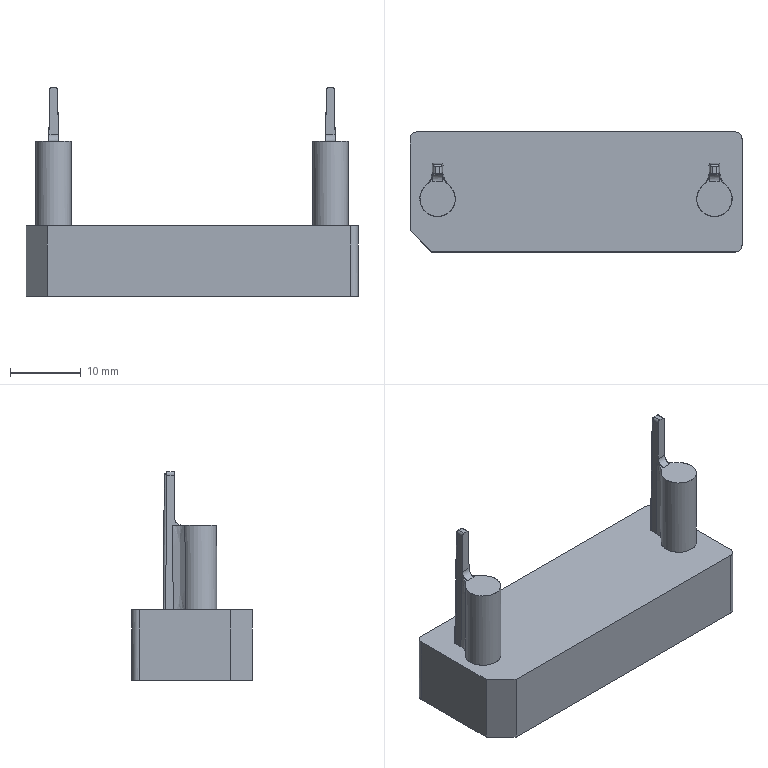NC program | PowerMill | posted with a generic post | part box 47 x 17 x 29.578 mm
Lines 10179 to 11327 of 293638:
N10276 M6
N10277 S8500 M03
N10278 G00 G90 X0.0 Y0.0
N10279 G43 Z11.798 H3
N10280
N10281 G05 P10000 R8
N10282 X-7.7871 Y4.8194
N10283 Z-6.65
N10284 G01 Z-7.85 F360.0
N10285 X-12.552 Y2.5562 F600.0
N10286 X-12.557 Y2.4789
N10287 X-12.5567 Y1.7113
N10288 X-12.567 Y1.1545
N10289 X-12.5886 Y0.8761
N10290 X-12.6226 Y0.5977
N10291 X-12.6693 Y0.3193
N10292 X-12.7485 Y-0.0401
N10293 X-12.813 Y-0.278
N10294 X-12.8876 Y-0.5159
N10295 X-12.988 Y-0.7943
N10296 X-13.1034 Y-1.0727
N10297 X-13.2152 Y-1.3105
N10298 X-13.297 Y-1.4712
N10299 X-13.3834 Y-1.6295
N10300 X-13.5505 Y-1.9079
N10301 X-13.7375 Y-2.1863
N10302 X-13.8817 Y-2.3809
N10303 X-14.0265 Y-2.562
N10304 X-14.1824 Y-2.7431
N10305 X-14.4483 Y-3.0228
N10306 X-14.7468 Y-3.2998
N10307 X-15.0149 Y-3.5209
N10308 X-15.2518 Y-3.6968
N10309 X-15.5815 Y-3.9151
N10310 X-15.8648 Y-4.0808
N10311 X-16.1481 Y-4.2269
N10312 X-16.57 Y-4.4134
N10313 X-16.7146 Y-4.4694
N10314 X-16.9979 Y-4.5672
N10315 X-17.2812 Y-4.6502
N10316 X-17.5645 Y-4.7196
N10317 X-17.8478 Y-4.7753
N10318 X-18.1311 Y-4.8177
N10319 X-18.4144 Y-4.8473
N10320 X-18.6977 Y-4.8644
N10321 X-18.981 Y-4.8688
N10322 X-19.2643 Y-4.8607
N10323 X-19.5477 Y-4.8408
N10324 X-20.1142 Y-4.8672
N10325 X-20.3975
N10326 X-20.6808 Y-4.8549
N10327 X-20.9641 Y-4.8299
N10328 X-21.2474 Y-4.7916
N10329 X-21.5307 Y-4.7406
N10330 X-21.814 Y-4.6763
N10331 X-22.0973 Y-4.598
N10332 X-22.3806 Y-4.5053
N10333 X-22.6252 Y-4.4134
N10334 X-22.9472 Y-4.2745
N10335 X-23.2305 Y-4.1342
N10336 X-23.5138 Y-3.9757
N10337 X-23.7057 Y-3.8571
N10338 X-23.8934 Y-3.732
N10339 X-24.0804 Y-3.597
N10340 X-24.2644 Y-3.454
N10341 X-24.4484 Y-3.2998
N10342 X-24.647 Y-3.1193
N10343 X-24.8375 Y-2.9312
N10344 X-25.0125 Y-2.7431
N10345 X-25.2136 Y-2.5071
N10346 X-25.4574 Y-2.1863
N10347 X-25.6273 Y-1.9352
N10348 X-25.7802 Y-1.6841
N10349 X-25.96 Y-1.3511
N10350 X-26.0915 Y-1.0727
N10351 X-26.207 Y-0.7943
N10352 X-26.3075 Y-0.5159
N10353 X-26.3468 Y-0.3944
N10354 X-26.4663 Y0.0409
N10355 X-26.5257 Y0.3193
N10356 X-26.5723 Y0.5977
N10357 X-26.6065 Y0.8761
N10358 X-26.6282 Y1.1545
N10359 X-26.6381 Y1.7113
N10360 X-26.6383 Y2.4181
N10361 X-26.6414 Y2.4792
N10362 X-26.6507 Y2.5398
N10363 G00 Z3.9981
N10364 G01 X-19.2742 Y-9.1382 F10000.0
N10365 G00 Z0.9281
N10366 G01 Z-0.2719 F360.0
N10367 Y-3.8632 F600.0
N10368 Y0.2836
N10369 G03 X-17.8374 Y1.7204 I0.0 J1.4368
N10370 G03 X-20.711 I-1.4368 J0.0
N10371 G03 X-19.2742 Y0.2836 I1.4368 J0.0
N10372 G01 Y-3.8632
N10373 G00 Z5.4237
N10374 G01 X31.4069 Y4.8215 F10000.0
N10375 G00 Z-6.65
N10376 G01 Z-7.85 F360.0
N10377 X26.643 Y2.5562 F600.0
N10378 X26.6381 Y2.4797
N10379 Y1.7113
N10380 X26.6282 Y1.1545
N10381 X26.6066 Y0.8761
N10382 X26.5723 Y0.5977
N10383 X26.5259 Y0.3193
N10384 X26.4663 Y0.0409
N10385 X26.3468 Y-0.3944
N10386 X26.2794 Y-0.5952
N10387 X26.2071 Y-0.7943
N10388 X26.0915 Y-1.0727
N10389 X25.9602 Y-1.3511
N10390 X25.7802 Y-1.6841
N10391 X25.6272 Y-1.9352
N10392 X25.4574 Y-2.1863
N10393 X25.2136 Y-2.5071
N10394 X25.0125 Y-2.7431
N10395 X24.8376 Y-2.9312
N10396 X24.647 Y-3.1193
N10397 X24.4484 Y-3.2998
N10398 X24.2644 Y-3.454
N10399 X24.0804 Y-3.597
N10400 G02 X23.5138 Y-3.9757 I-3.8683 J5.1742
N10401 G01 X23.2305 Y-4.1342
N10402 X22.9472 Y-4.2745
N10403 X22.6252 Y-4.4134
N10404 X22.3806 Y-4.5053
N10405 X22.0973 Y-4.598
N10406 X21.814 Y-4.6763
N10407 X21.5307 Y-4.7406
N10408 X21.2474 Y-4.7916
N10409 X20.9641 Y-4.8299
N10410 X20.6808 Y-4.8549
N10411 X20.3975 Y-4.8672
N10412 X20.1142
N10413 X19.5477 Y-4.8408
N10414 X19.2643 Y-4.8607
N10415 X18.981 Y-4.8688
N10416 X18.6977 Y-4.8644
N10417 X18.4144 Y-4.8473
N10418 X18.1311 Y-4.8177
N10419 X17.8478 Y-4.7753
N10420 X17.5645 Y-4.7196
N10421 X17.2812 Y-4.6502
N10422 X16.9979 Y-4.5672
N10423 X16.7146 Y-4.4694
N10424 X16.57 Y-4.4134
N10425 X16.1481 Y-4.2269
N10426 X15.8648 Y-4.0808
N10427 X15.5815 Y-3.9151
N10428 X15.2518 Y-3.6968
N10429 X15.0149 Y-3.5209
N10430 X14.7468 Y-3.2998
N10431 X14.4483 Y-3.0228
N10432 X14.1824 Y-2.7431
N10433 X14.0265 Y-2.562
N10434 X13.8817 Y-2.3809
N10435 X13.7375 Y-2.1863
N10436 X13.5502 Y-1.9079
N10437 X13.3834 Y-1.6295
N10438 X13.3151 Y-1.5052
N10439 X13.204 Y-1.289
N10440 X13.1034 Y-1.0727
N10441 X12.9877 Y-0.7943
N10442 X12.8876 Y-0.5159
N10443 X12.8129 Y-0.278
N10444 X12.7285 Y0.0409
N10445 X12.6693 Y0.3193
N10446 X12.6226 Y0.5977
N10447 X12.5887 Y0.8761
N10448 X12.567 Y1.1545
N10449 X12.5567 Y1.7113
N10450 X12.5568 Y2.4176
N10451 X12.5537 Y2.479
N10452 X12.5443 Y2.5398
N10453 G00 Z3.9981
N10454 G01 X29.3429 Y-4.3729 F10000.0
N10455 G00 Z0.9281
N10456 G01 Z-0.2719 F360.0
N10457 X25.0882 Y-1.2546 F600.0
N10458 X21.6567 Y1.319
N10459 G03 X21.97 Y2.2589 I-1.2531 J0.9399
N10460 G03 X18.8371 I-1.5665 J0.0
N10461 G03 X21.6567 Y1.319 I1.5664 J0.0
N10462 G01 X25.0882 Y-1.2546
N10463 G00 Z11.798
N10464 G05 P0
N10465 (---------------)
N10466 ( END TOOLPATH : 精公基准台01-平坦面偏置-D10 )
N10467 (---------------)
N10468 ( START TOOLPATH : 精公基准台01-基准面偏置-D10 )
N10469 (---------------)
N10470 G00 X0.0 Y0.0 Z9.7981
N10471 G05 P10000 R8
N10472 X34.16 Y-0.7311
N10473 Z-18.58
N10474 G01 Z-19.78 F360.0
N10475 X28.885 Y-0.7312 F600.0
N10476 X27.474 Y-0.7792
N10477 X27.4764 Y-1.1334
N10478 X27.4657 Y-1.4167
N10479 X27.4449 Y-1.7001
N10480 X27.414 Y-1.9834
N10481 X27.3726 Y-2.2667
N10482 X27.3202 Y-2.5501
N10483 X27.2581 Y-2.8305
N10484 X27.1833 Y-3.1168
N10485 X27.0977 Y-3.4001
N10486 X27.0005 Y-3.6834
N10487 X26.8914 Y-3.9668
N10488 X26.7688 Y-4.2501
N10489 X26.6184 Y-4.562
N10490 X26.4826 Y-4.8168
N10491 X26.317 Y-5.1002
N10492 X26.135 Y-5.3835
N10493 X26.052 Y-5.5044
N10494 X25.8899 Y-5.7273
N10495 X25.7157 Y-5.9502
N10496 X25.4857 Y-6.2202
N10497 X25.349 Y-6.3705
N10498 X25.2083 Y-6.5169
N10499 X24.9193 Y-6.7955
N10500 X24.5864 Y-7.0836
N10501 X24.353 Y-7.2673
N10502 X24.0746 Y-7.4686
N10503 X23.7866 Y-7.6583
N10504 X23.5035 Y-7.8279
N10505 X23.2203 Y-7.982
N10506 X22.97 Y-8.106
N10507 X22.6539 Y-8.2471
N10508 X22.3708 Y-8.3601
N10509 X22.0876 Y-8.4604
N10510 X21.8044 Y-8.5488
N10511 X21.5212 Y-8.6256
N10512 X21.2381 Y-8.6914
N10513 X20.9549 Y-8.7462
N10514 X20.7201 Y-8.7836
N10515 X20.3885 Y-8.8243
N10516 X20.1054 Y-8.8477
N10517 X19.8222 Y-8.8605
N10518 X19.539 Y-8.8638
N10519 X19.2558 Y-8.8567
N10520 X18.9727 Y-8.8393
N10521 X18.6895 Y-8.8116
N10522 X18.4749 Y-8.7836
N10523 X18.1231 Y-8.7247
N10524 X17.84 Y-8.6656
N10525 X17.5568 Y-8.5952
N10526 X17.2736 Y-8.5135
N10527 X16.9904 Y-8.4203
N10528 X16.7305 Y-8.3237
N10529 X16.4241 Y-8.1967
N10530 X16.1409 Y-8.0654
N10531 X15.8578 Y-7.92
N10532 X15.6267 Y-7.7903
N10533 X15.2914 Y-7.5833
N10534 X15.0082 Y-7.3898
N10535 X14.7251 Y-7.1771
N10536 X14.6086 Y-7.0836
N10537 X14.3837 Y-6.8925
N10538 X14.1587 Y-6.6862
N10539 X13.9867 Y-6.5169
N10540 X13.7822 Y-6.3016
N10541 X13.5924 Y-6.0863
N10542 X13.4793 Y-5.9502
N10543 X13.2599 Y-5.6668
N10544 X13.026 Y-5.3326
N10545 X12.8625 Y-5.0747
N10546 X12.7124 Y-4.8168
N10547 X12.5802 Y-4.5692
N10548 X12.4265 Y-4.2501
N10549 X12.3035 Y-3.9668
N10550 X12.1953 Y-3.6834
N10551 X12.0971 Y-3.4001
N10552 X12.0114 Y-3.1168
N10553 X11.8933 Y-2.6392
N10554 X11.8222 Y-2.2667
N10555 X11.781 Y-1.9834
N10556 X11.7498 Y-1.7001
N10557 X11.7293 Y-1.4167
N10558 X11.7189 Y-1.1334
N10559 X11.7185 Y-0.85
N10560 X11.7487 Y-0.2833
N10561 X11.779 Y0.0
N10562 X11.82 Y0.2833
N10563 X11.8933 Y0.6713
N10564 X11.9337 Y0.85
N10565 X12.0073 Y1.1334
N10566 X12.0919 Y1.4167
N10567 X12.1886 Y1.7001
N10568 X12.2973 Y1.9834
N10569 X12.3693 Y2.148
N10570 G03 X12.453 Y2.5501 I-0.9163 J0.4006
N10571 G01 X12.4503 Y3.6834
N10572 X12.4597 Y4.1774
N10573 X12.4899 Y4.5335
N10574 X12.5288 Y4.8168
N10575 X12.5806 Y5.1002
N10576 X12.643 Y5.3835
N10577 X12.7183 Y5.6668
N10578 X12.8081 Y5.9502
N10579 X12.9094 Y6.2259
N10580 X13.0329 Y6.5169
N10581 X13.1682 Y6.8002
N10582 X13.3189 Y7.0836
N10583 X13.4495 Y7.3046
N10584 X13.5924 Y7.5257
N10585 X13.6789 Y7.6502
N10586 X13.8923 Y7.9336
N10587 X14.1587 Y8.249
N10588 X14.4265 Y8.5321
N10589 X14.7251 Y8.8104
N10590 X15.0082 Y9.0443
N10591 X15.2914 Y9.2529
N10592 X15.4324 Y9.3503
N10593 X15.6451 Y9.4869
N10594 X15.8578 Y9.612
N10595 X16.1409 Y9.7622
N10596 X16.4758 Y9.917
N10597 X16.9904 Y10.1154
N10598 X17.2736 Y10.205
N10599 X17.5568 Y10.2803
N10600 X17.84 Y10.3418
N10601 X18.1231 Y10.3904
N10602 X18.4063 Y10.427
N10603 X18.6895 Y10.4529
N10604 X18.9727 Y10.4661
N10605 X19.8222 Y10.4682
N10606 X20.3885 Y10.4599
N10607 X20.6717 Y10.439
N10608 X20.9549 Y10.4065
N10609 X21.2381 Y10.3634
N10610 X21.5212 Y10.3074
N10611 X21.8044 Y10.2378
N10612 X22.0876 Y10.1541
N10613 X22.3708 Y10.0559
N10614 X22.7192 Y9.917
N10615 X22.9697 Y9.8034
N10616 X23.2203 Y9.6762
N10617 X23.4914 Y9.5226
N10618 X23.7866 Y9.3342
N10619 X24.0698 Y9.1329
N10620 X24.353 Y8.9103
N10621 X24.5006 Y8.7836
N10622 X24.71 Y8.5895
N10623 X24.9193 Y8.3769
N10624 X25.0648 Y8.2169
N10625 X25.2854 Y7.9549
N10626 X25.5161 Y7.6502
N10627 X25.7069 Y7.3669
N10628 X25.8761 Y7.0836
N10629 X26.052 Y6.7485
N10630 X26.1621 Y6.5169
N10631 X26.2826 Y6.2335
N10632 X26.3869 Y5.9502
N10633 X26.4765 Y5.6668
N10634 X26.552 Y5.3835
N10635 X26.6184 Y5.0802
N10636 X26.6662 Y4.8168
N10637 X26.7049 Y4.5335
N10638 X26.7309 Y4.2501
N10639 X26.744 Y3.9668
N10640 X26.742 Y2.554
N10641 G03 X26.8223 Y2.1598 I1.0 J-0.0015
N10642 G01 X26.8977 Y1.9834
N10643 X27.0067 Y1.7001
N10644 X27.1031 Y1.4167
N10645 X27.1847 Y1.1442
N10646 X27.261 Y0.85
N10647 X27.3234 Y0.5667
N10648 X27.375 Y0.2833
N10649 X27.4159 Y0.0
N10650 X27.4463 Y-0.2833
N10651 X27.4668 Y-0.5667
N10652 X27.474 Y-0.7792
N10653 X28.885 Y-0.7312
N10654 G00 Z2.8214
N10655 G01 X-34.16 Y-1.292 F10000.0
N10656 G00 Z-18.58
N10657 G01 Z-19.78 F360.0
N10658 X-28.885 F600.0
N10659 X-27.4722 Y-1.2396
N10660 X-27.4762 Y-1.1334
N10661 X-27.4765 Y-0.85
N10662 X-27.4463 Y-0.2833
N10663 X-27.416 Y0.0
N10664 X-27.375 Y0.2833
N10665 X-27.3236 Y0.5667
N10666 X-27.2613 Y0.85
N10667 X-27.1847 Y1.1439
N10668 X-27.1031 Y1.4167
N10669 X-27.0063 Y1.7001
N10670 X-26.8977 Y1.9834
N10671 X-26.8231 Y2.1571
N10672 G03 X-26.742 Y2.5531 I-0.9189 J0.3945
N10673 G01 X-26.7442 Y3.9668
N10674 X-26.7309 Y4.2501
N10675 X-26.705 Y4.5335
N10676 X-26.6662 Y4.8168
N10677 X-26.6184 Y5.0802
N10678 X-26.552 Y5.3835
N10679 X-26.4766 Y5.6668
N10680 X-26.3869 Y5.9502
N10681 X-26.2825 Y6.2335
N10682 X-26.1621 Y6.5169
N10683 X-26.052 Y6.7485
N10684 X-25.8761 Y7.0836
N10685 X-25.7068 Y7.3669
N10686 X-25.4857 Y7.6928
N10687 X-25.2855 Y7.9549
N10688 X-25.0648 Y8.2169
N10689 X-24.9193 Y8.3769
N10690 X-24.71 Y8.5895
N10691 X-24.5006 Y8.7836
N10692 X-24.353 Y8.9103
N10693 X-24.0698 Y9.1329
N10694 X-23.7626 Y9.3503
N10695 X-23.4914 Y9.5226
N10696 X-23.2203 Y9.6762
N10697 X-22.9697 Y9.8034
N10698 X-22.6539 Y9.9446
N10699 X-22.3708 Y10.0559
N10700 X-22.0876 Y10.1541
N10701 X-21.8044 Y10.2378
N10702 X-21.5212 Y10.3074
N10703 X-21.2381 Y10.3634
N10704 X-20.9549 Y10.4065
N10705 X-20.6717 Y10.439
N10706 X-20.3885 Y10.4599
N10707 X-19.8222 Y10.4682
N10708 X-18.9727 Y10.4661
N10709 X-18.6895 Y10.4529
N10710 X-18.4063 Y10.427
N10711 X-18.1231 Y10.3904
N10712 X-17.84 Y10.3418
N10713 X-17.5568 Y10.2803
N10714 X-17.2736 Y10.205
N10715 X-16.9904 Y10.1154
N10716 X-16.4241 Y9.8946
N10717 X-16.1409 Y9.7622
N10718 X-15.8578 Y9.612
N10719 X-15.6451 Y9.4869
N10720 X-15.4324 Y9.3503
N10721 X-15.2914 Y9.2529
N10722 X-15.0082 Y9.0443
N10723 X-14.6944 Y8.7836
N10724 X-14.4265 Y8.5321
N10725 X-14.1302 Y8.2169
N10726 X-13.8925 Y7.9336
N10727 X-13.6789 Y7.6502
N10728 X-13.5924 Y7.5257
N10729 X-13.4493 Y7.3046
N10730 X-13.3189 Y7.0836
N10731 X-13.1685 Y6.8002
N10732 X-13.026 Y6.5016
N10733 X-12.9097 Y6.2259
N10734 X-12.8081 Y5.9502
N10735 X-12.7185 Y5.6668
N10736 X-12.643 Y5.3835
N10737 X-12.5806 Y5.1002
N10738 X-12.5288 Y4.8168
N10739 X-12.49 Y4.5335
N10740 X-12.4597 Y4.1774
N10741 X-12.4503 Y3.6834
N10742 X-12.453 Y2.5501
N10743 G03 X-12.3693 Y2.148 I1.0 J-0.0015
N10744 G01 X-12.2973 Y1.9834
N10745 X-12.1887 Y1.7001
N10746 X-12.0919 Y1.4167
N10747 X-12.0073 Y1.1334
N10748 X-11.9337 Y0.85
N10749 X-11.8933 Y0.6713
N10750 X-11.82 Y0.2833
N10751 X-11.7793 Y0.0
N10752 X-11.7487 Y-0.2833
N10753 X-11.7391 Y-0.417
N10754 X-2.1427 Y0.1223
N10755 G02 X-2.1615 Y-2.3231 I-19.141 J-1.0756
N10756 G01 X-2.2157 Y-3.0789
N10757 G03 X-1.1028 Y-4.2743 I1.1129 J-0.0797
N10758 G01 X1.1043
N10759 G03 X2.2173 Y-3.0836 I-0.0001 J1.1156
N10760 G01 X2.155 Y-2.16
N10761 G02 X2.1691 Y0.3517 I17.1882 J1.1596
N10762 G01 X2.2059 Y0.7628
N10763 X2.529 Y2.9746
N10764 G03 X1.4055 Y4.2741 I-1.1234 J0.1641
N10765 G01 X-1.4052
N10766 G03 X-2.509 Y2.9462 I0.0 J-1.1227
N10767 G01 X-2.4354 Y2.5501
N10768 G02 X-2.1427 Y0.1223 I-18.8484 J-3.5034
N10769 G01 X-6.9409 Y-0.1474
N10770 G03 X-7.0715 Y1.0301 I-12.7751 J-0.8208
N10771 G01 X-7.7871 Y5.5581
N10772 G03 X-8.1764 Y7.2141 I-11.337 J-1.7916
N10773 G01 X-8.4118 Y7.9616
N10774 G02 X-7.5921 Y9.0792 I0.8198 J0.2581
N10775 G01 X7.5917 Y9.0796
N10776 G02 X8.406 Y7.9468 I0.0 J-0.8591
N10777 G01 X8.2989 Y7.6281
N10778 G03 X7.7656 Y5.4429 I12.5815 J-4.2282
N10779 G01 X7.0226 Y0.6418
N10780 X6.979 Y0.2501
N10781 G03 X8.646 Y-7.371 I12.575 J-1.2423
N10782 G01 X9.0108 Y-7.9949
N10783 G02 X8.3887 Y-9.0794 I-0.6221 J-0.3638
N10784 G01 X-8.3884 Y-9.0798
N10785 G02 X-9.0011 Y-7.9806 I0.0 J0.7203
N10786 G01 X-8.8281 Y-7.7008
N10787 G03 X-6.9409 Y-0.1474 I-10.8879 J6.7326
N10788 G01 X-11.7391 Y-0.417
N10789 X-11.7284 Y-0.5667
N10790 X-11.7185 Y-0.85
N10791 X-11.7188 Y-1.1334
N10792 X-11.7293 Y-1.4167
N10793 X-11.7499 Y-1.7001
N10794 X-11.781 Y-1.9834
N10795 X-11.8225 Y-2.2667
N10796 X-11.8933 Y-2.6392
N10797 X-12.0114 Y-3.1168
N10798 X-12.0973 Y-3.4001
N10799 X-12.1947 Y-3.6834
N10800 X-12.3036 Y-3.9668
N10801 X-12.4597 Y-4.3226
N10802 X-12.579 Y-4.5671
N10803 X-12.7124 Y-4.8168
N10804 X-12.8624 Y-5.0747
N10805 X-13.06 Y-5.3835
N10806 X-13.2599 Y-5.6668
N10807 X-13.4793 Y-5.9502
N10808 X-13.5924 Y-6.086
N10809 X-13.7811 Y-6.3005
N10810 X-13.9864 Y-6.5169
N10811 X-14.1587 Y-6.6862
N10812 X-14.3852 Y-6.8938
N10813 X-14.6086 Y-7.0836
N10814 X-14.7251 Y-7.1771
N10815 X-15.0082 Y-7.3898
N10816 X-15.2914 Y-7.5835
N10817 X-15.6267 Y-7.7903
N10818 X-15.8578 Y-7.92
N10819 X-16.1409 Y-8.0654
N10820 X-16.4706 Y-8.2169
N10821 X-16.7305 Y-8.324
N10822 X-16.9904 Y-8.4203
N10823 X-17.2736 Y-8.5135
N10824 X-17.5568 Y-8.5952
N10825 X-17.84 Y-8.6656
N10826 X-18.1231 Y-8.7249
N10827 X-18.4749 Y-8.7836
N10828 X-18.6895 Y-8.8116
N10829 X-18.9727 Y-8.839
N10830 X-19.2558 Y-8.8567
N10831 X-19.539 Y-8.8638
N10832 X-19.8222 Y-8.8605
N10833 X-20.1054 Y-8.8477
N10834 X-20.3885 Y-8.8243
N10835 X-20.7201 Y-8.7836
N10836 X-20.9549 Y-8.7462
N10837 X-21.2381 Y-8.6914
N10838 X-21.5212 Y-8.6256
N10839 X-21.8044 Y-8.5488
N10840 X-22.0876 Y-8.4601
N10841 X-22.3708 Y-8.3601
N10842 X-22.7247 Y-8.2169
N10843 X-22.9725 Y-8.1047
N10844 X-23.2203 Y-7.982
N10845 X-23.5035 Y-7.8279
N10846 X-23.7993 Y-7.6502
N10847 X-24.0762 Y-7.4676
N10848 X-24.353 Y-7.2673
N10849 X-24.5864 Y-7.0836
N10850 X-24.9193 Y-6.7955
N10851 X-25.2083 Y-6.5169
N10852 X-25.4857 Y-6.2208
N10853 X-25.7157 Y-5.9502
N10854 X-25.8902 Y-5.7273
N10855 X-26.052 Y-5.5044
N10856 X-26.135 Y-5.3835
N10857 X-26.3172 Y-5.1002
N10858 X-26.4826 Y-4.8168
N10859 X-26.6184 Y-4.562
N10860 X-26.7688 Y-4.2501
N10861 X-26.8912 Y-3.9668
N10862 X-27.0005 Y-3.6834
N10863 X-27.0976 Y-3.4001
N10864 X-27.1836 Y-3.1168
N10865 X-27.2581 Y-2.8311
N10866 X-27.3205 Y-2.5501
N10867 X-27.3725 Y-2.2667
N10868 X-27.414 Y-1.9834
N10869 X-27.4451 Y-1.7001
N10870 X-27.4657 Y-1.4167
N10871 X-27.4722 Y-1.2396
N10872 X-28.885 Y-1.292
N10873 G00 Z9.7981
N10874 G05 P0
N10875 (---------------)
N10876 ( END TOOLPATH : 精公基准台01-基准面偏置-D10 )
N10877 (---------------)
N10878 ( START TOOLPATH : 精公基准台01-基准台侧光-D10 )
N10879 (---------------)
N10880 G00 X0.0 Y0.0 Z9.7981
N10881 G05 P10000 R8
N10882 X28.7181 Y-16.6674
N10883 Z-28.48
N10884 G01 Z-29.68 F360.0
N10885 G03 X25.8667 Y-12.5602 I-1.4257 J2.0536 F600.0
N10886 G01 X25.8115 Y-12.5985
N10887 X25.8099 Y-12.5996
N10888 X25.8083 Y-12.6006
N10889 X25.6279 Y-12.7136
N10890 X25.6268 Y-12.7143
N10891 X25.6257 Y-12.715
N10892 X25.49 Y-12.7939
N10893 X25.4885 Y-12.7948
N10894 X25.487 Y-12.7956
N10895 X25.1708 Y-12.9619
N10896 X25.1693 Y-12.9627
N10897 X25.1677 Y-12.9635
N10898 X25.0174 Y-13.0343
N10899 X25.0164 Y-13.0348
N10900 X25.0153 Y-13.0353
N10901 X24.8494 Y-13.1077
N10902 X24.8478 Y-13.1084
N10903 X24.8462 Y-13.109
N10904 X24.5301 Y-13.231
N10905 X24.5278 Y-13.2319
N10906 X24.5254 Y-13.2326
N10907 X24.1404 Y-13.3544
N10908 X24.1384 Y-13.355
N10909 X24.1363 Y-13.3556
N10910 X23.8889 Y-13.4192
N10911 X23.887 Y-13.4197
N10912 X23.885 Y-13.4201
N10913 X23.5688 Y-13.4846
N10914 X23.5669 Y-13.485
N10915 X23.5649 Y-13.4853
N10916 X23.2488 Y-13.5337
N10917 X23.2465 Y-13.534
N10918 X23.2443 Y-13.5342
N10919 X22.9281 Y-13.5642
N10920 X22.9262 Y-13.5644
N10921 X22.9242 Y-13.5645
N10922 X22.608 Y-13.5788
N10923 X22.6064 Y-13.5789
N10924 X22.6047
N10925 X22.2885 Y-13.58
N10926 X22.2884
N10927 X22.2883
N10928 X-20.3914
N10929 X-20.3919
N10930 X-20.3925
N10931 X-20.7086 Y-13.5757
N10932 X-20.711 Y-13.5756
N10933 X-20.7134 Y-13.5755
N10934 X-21.0295 Y-13.5523
N10935 X-21.0321 Y-13.5521
N10936 X-21.0346 Y-13.5518
N10937 X-21.3507 Y-13.5082
N10938 X-21.3533 Y-13.5078
N10939 X-21.3558 Y-13.5074
N10940 X-21.672 Y-13.4429
N10941 X-21.6745 Y-13.4424
N10942 X-21.677 Y-13.4417
N10943 X-21.9932 Y-13.3556
N10944 X-21.9957 Y-13.3548
N10945 X-21.9982 Y-13.354
N10946 X-22.3144 Y-13.2449
N10947 X-22.3169 Y-13.244
N10948 X-22.3194 Y-13.243
N10949 X-22.6356 Y-13.1093
N10950 X-22.6375 Y-13.1084
N10951 X-22.6393 Y-13.1076
N10952 X-22.7912 Y-13.034
N10953 X-22.7924 Y-13.0333
N10954 X-22.7937 Y-13.0327
N10955 X-22.958 Y-12.9458
N10956 X-22.9599 Y-12.9447
N10957 X-22.9618 Y-12.9436
N10958 X-23.278 Y-12.7531
N10959 X-23.2806 Y-12.7515
N10960 X-23.2831 Y-12.7498
N10961 X-23.5992 Y-12.525
N10962 X-23.6011 Y-12.5236
N10963 X-23.603 Y-12.5221
N10964 X-23.7647 Y-12.392
N10965 X-23.766 Y-12.391
N10966 X-23.7673 Y-12.3899
N10967 X-23.9217 Y-12.2548
N10968 X-23.9231 Y-12.2535
N10969 X-23.9244 Y-12.2523
N10970 X-24.113 Y-12.0712
N10971 X-24.1135 Y-12.0707
N10972 X-24.1141 Y-12.0701
N10973 X-27.087 Y-9.0972
N10974 X-27.0877 Y-9.0965
N10975 X-27.0884 Y-9.0958
N10976 X-27.2679 Y-8.9072
N10977 X-27.2692 Y-8.9059
N10978 X-27.2704 Y-8.9045
N10979 X-27.4071 Y-8.7467
N10980 X-27.4081 Y-8.7454
N10981 X-27.4092 Y-8.7442
N10982 X-27.5354 Y-8.5858
N10983 X-27.5367 Y-8.5841
N10984 X-27.5379 Y-8.5824
N10985 X-27.7279 Y-8.3162
N10986 X-27.7296 Y-8.3137
N10987 X-27.7312 Y-8.3112
N10988 X-27.9528 Y-7.9451
N10989 X-27.9541 Y-7.9429
N10990 X-27.9553 Y-7.9407
N10991 X-28.0498 Y-7.7595
N10992 X-28.0505 Y-7.7583
N10993 X-28.0511 Y-7.757
N10994 X-28.1156 Y-7.622
N10995 X-28.1164 Y-7.6202
N10996 X-28.1172 Y-7.6184
N10997 X-28.2495 Y-7.3022
N10998 X-28.2505 Y-7.2997
N10999 X-28.2514 Y-7.2972
N11000 X-28.3593 Y-6.981
N11001 X-28.3601 Y-6.9785
N11002 X-28.3608 Y-6.976
N11003 X-28.4458 Y-6.6598
N11004 X-28.4464 Y-6.6573
N11005 X-28.447 Y-6.6548
N11006 X-28.5103 Y-6.3386
N11007 X-28.5107 Y-6.3361
N11008 X-28.5111 Y-6.3336
N11009 X-28.5535 Y-6.0174
N11010 X-28.5538 Y-6.0149
N11011 X-28.5541 Y-6.0124
N11012 X-28.5762 Y-5.6962
N11013 X-28.5763 Y-5.6939
N11014 X-28.5764 Y-5.6915
N11015 X-28.58 Y-5.3754
N11016 Y-5.3749
N11017 Y-5.3745
N11018 X-28.5792 Y7.5875
N11019 Y7.5891
N11020 Y7.5907
N11021 X-28.5663 Y7.9069
N11022 X-28.5662 Y7.909
N11023 X-28.5661 Y7.9111
N11024 X-28.5363 Y8.2273
N11025 X-28.536 Y8.2294
N11026 X-28.5358 Y8.2315
N11027 X-28.489 Y8.5476
N11028 X-28.4887 Y8.5498
N11029 X-28.4883 Y8.5519
N11030 X-28.424 Y8.868
N11031 X-28.4236 Y8.8701
N11032 X-28.423 Y8.8722
N11033 X-28.3407 Y9.1884
N11034 X-28.3402 Y9.1905
N11035 X-28.3395 Y9.1926
N11036 X-28.2384 Y9.5087
N11037 X-28.2377 Y9.5108
N11038 X-28.2369 Y9.5129
N11039 X-28.1162 Y9.8291
N11040 X-28.1156 Y9.8306
N11041 X-28.1149 Y9.8322
N11042 X-28.0524 Y9.9774
N11043 X-28.0519 Y9.9785
N11044 X-28.0514 Y9.9796
N11045 X-27.9717 Y10.1505
N11046 X-27.9709 Y10.1521
N11047 X-27.9701 Y10.1537
N11048 X-27.8052 Y10.4698
N11049 X-27.8044 Y10.4713
N11050 X-27.8036 Y10.4727
N11051 X-27.7321 Y10.5969
N11052 X-27.7314 Y10.598
N11053 X-27.7308 Y10.5991
N11054 X-27.6121 Y10.791
N11055 X-27.6111 Y10.7926
N11056 X-27.61 Y10.7942
N11057 X-27.4126 Y11.0822
N11058 X-27.4111 Y11.0844
N11059 X-27.4095 Y11.0865
N11060 X-27.1384 Y11.4307
N11061 X-27.1366 Y11.433
N11062 X-27.1347 Y11.4351
N11063 X-26.8465 Y11.7513
N11064 X-26.8453 Y11.7526
N11065 X-26.844 Y11.7538
N11066 X-26.771 Y11.8272
N11067 X-26.7699 Y11.8283
N11068 X-26.7688 Y11.8293
N11069 X-26.5075 Y12.0721
N11070 X-26.5055 Y12.074
N11071 X-26.5033 Y12.0758
N11072 X-26.1323 Y12.3756
N11073 X-26.13 Y12.3774
N11074 X-26.1276 Y12.3791
N11075 X-25.8115 Y12.5985
N11076 X-25.8099 Y12.5996
N11077 X-25.8083 Y12.6006
N11078 X-25.6279 Y12.7136
N11079 X-25.6268 Y12.7143
N11080 X-25.6257 Y12.715
N11081 X-25.49 Y12.7939
N11082 X-25.4885 Y12.7948
N11083 X-25.487 Y12.7956
N11084 X-25.1708 Y12.9619
N11085 X-25.1693 Y12.9627
N11086 X-25.1677 Y12.9635
N11087 X-25.0174 Y13.0343
N11088 X-25.0164 Y13.0348
N11089 X-25.0153 Y13.0353
N11090 X-24.8494 Y13.1077
N11091 X-24.8478 Y13.1084
N11092 X-24.8462 Y13.109
N11093 X-24.5301 Y13.231
N11094 X-24.528 Y13.2318
N11095 X-24.5259 Y13.2325
N11096 X-24.2097 Y13.3346
N11097 X-24.2076 Y13.3353
N11098 X-24.2055 Y13.3359
N11099 X-23.8894 Y13.4191
N11100 X-23.8872 Y13.4196
N11101 X-23.885 Y13.4201
N11102 X-23.5688 Y13.4846
N11103 X-23.5669 Y13.485
N11104 X-23.5649 Y13.4853
N11105 X-23.2488 Y13.5337
N11106 X-23.2465 Y13.534
N11107 X-23.2443 Y13.5342
N11108 X-22.9281 Y13.5642
N11109 X-22.9262 Y13.5644
N11110 X-22.9242 Y13.5645
N11111 X-22.608 Y13.5788
N11112 X-22.6064 Y13.5789
N11113 X-22.6047
N11114 X-22.2885 Y13.58
N11115 X-22.2884
N11116 X-22.2883
N11117 X0.0
N11118 X22.2883
N11119 X22.2884
N11120 X22.2885
N11121 X22.6047 Y13.5789
N11122 X22.6063
N11123 X22.6079 Y13.5788
N11124 X22.924 Y13.5652
N11125 X22.9262 Y13.565
N11126 X22.9283 Y13.5649
N11127 X23.2444 Y13.5342
N11128 X23.2465 Y13.534
N11129 X23.2486 Y13.5337
N11130 X23.5648 Y13.486
N11131 X23.5669 Y13.4857
N11132 X23.569 Y13.4853
N11133 X23.8852 Y13.4201
N11134 X23.887 Y13.4197
N11135 X23.8889 Y13.4192
N11136 X24.1362 Y13.3556
N11137 X24.1384 Y13.355
N11138 X24.1405 Y13.3544
N11139 X24.5255 Y13.2324
N11140 X24.5278 Y13.2317
N11141 X24.53 Y13.2308
N11142 X24.8462 Y13.109
N11143 X24.8478 Y13.1084
N11144 X24.8495 Y13.1077
N11145 X25.0153 Y13.0353
N11146 X25.0164 Y13.0348
N11147 X25.0175 Y13.0343
N11148 X25.1678 Y12.9632
N11149 X25.1693 Y12.9624
N11150 X25.1708 Y12.9617
N11151 X25.4869 Y12.7956
N11152 X25.4885 Y12.7948
N11153 X25.49 Y12.7939
N11154 X25.6257 Y12.715
N11155 X25.6267 Y12.7143
N11156 X25.6278 Y12.7137
N11157 X25.8082 Y12.601
N11158 X25.8098 Y12.6
N11159 X25.8114 Y12.599
N11160 X26.1055 Y12.3955
N11161 X26.1077 Y12.3939
N11162 X26.1098 Y12.3923
N11163 X26.4479 Y12.1238
N11164 X26.4501 Y12.1219
N11165 X26.4523 Y12.12
N11166 X26.7684 Y11.8297
N11167 X26.7697 Y11.8284
N11168 X26.771 Y11.8272
N11169 X26.844 Y11.7538
N11170 X26.8451 Y11.7527
N11171 X26.8462 Y11.7516
N11172 X27.0893 Y11.4878
N11173 X27.0911 Y11.4857
N11174 X27.0929 Y11.4836
N11175 X27.3883 Y11.1152
N11176 X27.3901 Y11.1129
N11177 X27.3918 Y11.1105
N11178 X27.6098 Y10.7944
N11179 X27.6108 Y10.7927
N11180 X27.6119 Y10.7911
N11181 X27.7308 Y10.5991
N11182 X27.7314 Y10.598
N11183 X27.7321 Y10.5969
N11184 X27.8036 Y10.4727
N11185 X27.8044 Y10.4713
N11186 X27.8052 Y10.4698
N11187 X27.9703 Y10.1537
N11188 X27.9713 Y10.1516
N11189 X27.9723 Y10.1495
N11190 X28.1144 Y9.8333
N11191 X28.1153 Y9.8312
N11192 X28.1162 Y9.8291
N11193 X28.237 Y9.5129
N11194 X28.2378 Y9.5108
N11195 X28.2385 Y9.5087
N11196 X28.3396 Y9.1926
N11197 X28.3402 Y9.1905
N11198 X28.3408 Y9.1884
N11199 X28.4231 Y8.8722
N11200 X28.4236 Y8.87
N11201 X28.4241 Y8.8678
N11202 X28.4876 Y8.5517
N11203 X28.488 Y8.5497
N11204 X28.4883 Y8.5478
N11205 X28.5357 Y8.2317
N11206 X28.536 Y8.2294
N11207 X28.5363 Y8.2271
N11208 X28.5653 Y7.911
N11209 X28.5655 Y7.909
N11210 X28.5656 Y7.9071
N11211 X28.5792 Y7.5909
N11212 Y7.5892
N11213 X28.5793 Y7.5875
N11214 X28.5792 Y-7.5875
N11215 Y-7.5891
N11216 Y-7.5907
N11217 X28.5663 Y-7.9069
N11218 X28.5662 Y-7.909
N11219 X28.5661 Y-7.9111
N11220 X28.5363 Y-8.2273
N11221 X28.536 Y-8.2294
N11222 X28.5358 Y-8.2315
N11223 X28.489 Y-8.5476
N11224 X28.4887 Y-8.5498
N11225 X28.4883 Y-8.5519
N11226 X28.424 Y-8.868
N11227 X28.4236 Y-8.8701
N11228 X28.423 Y-8.8722
N11229 X28.3407 Y-9.1884
N11230 X28.3402 Y-9.1905
N11231 X28.3395 Y-9.1926
N11232 X28.2384 Y-9.5087
N11233 X28.2377 Y-9.5108
N11234 X28.2369 Y-9.5129
N11235 X28.1162 Y-9.8291
N11236 X28.1156 Y-9.8306
N11237 X28.1149 Y-9.8322
N11238 X28.0524 Y-9.9774
N11239 X28.0519 Y-9.9785
N11240 X28.0514 Y-9.9796
N11241 X27.9717 Y-10.1505
N11242 X27.9709 Y-10.1521
N11243 X27.9701 Y-10.1537
N11244 X27.8052 Y-10.4698
N11245 X27.8044 Y-10.4713
N11246 X27.8036 Y-10.4727
N11247 X27.7321 Y-10.5969
N11248 X27.7314 Y-10.598
N11249 X27.7308 Y-10.5991
N11250 X27.6121 Y-10.791
N11251 X27.6111 Y-10.7926
N11252 X27.61 Y-10.7942
N11253 X27.4126 Y-11.0822
N11254 X27.4111 Y-11.0844
N11255 X27.4095 Y-11.0865
N11256 X27.1384 Y-11.4307
N11257 X27.1366 Y-11.433
N11258 X27.1347 Y-11.4351
N11259 X26.8465 Y-11.7513
N11260 X26.8453 Y-11.7526
N11261 X26.844 Y-11.7538
N11262 X26.771 Y-11.8272
N11263 X26.7699 Y-11.8283
N11264 X26.7688 Y-11.8293
N11265 X26.5075 Y-12.0721
N11266 X26.5055 Y-12.074
N11267 X26.5033 Y-12.0758
N11268 X26.1323 Y-12.3756
N11269 X26.13 Y-12.3774
N11270 X26.1276 Y-12.3791
N11271 X25.8667 Y-12.5602
N11272 G03 X28.7181 Y-16.6675 I1.4257 J-2.0537
N11273 G01 X28.6676 Y-16.6052
N11274 G03 X25.8161 Y-12.498 I-1.4258 J2.0536
N11275 G01 X25.7659 Y-12.5328
N11276 X25.5854 Y-12.6458
N11277 X25.4497 Y-12.7248
N11278 X25.1336 Y-12.8911
N11279 X24.9833 Y-12.962
N11280 X24.8174 Y-13.0344
N11281 X24.5013 Y-13.1564
N11282 X24.1163 Y-13.2781
N11283 X23.869 Y-13.3417
N11284 X23.5529 Y-13.4062
N11285 X23.2367 Y-13.4546
N11286 X22.9206 Y-13.4846
N11287 X22.6044 Y-13.4989
N11288 X22.2883 Y-13.5
N11289 X-20.3914
N11290 X-20.7075 Y-13.4957
N11291 X-21.0237 Y-13.4725
N11292 X-21.3398 Y-13.429
N11293 X-21.656 Y-13.3645
N11294 X-21.9721 Y-13.2784
N11295 X-22.2883 Y-13.1693
N11296 X-22.6044 Y-13.0356
N11297 X-22.7563 Y-12.962
N11298 X-22.9206 Y-12.875
N11299 X-23.2367 Y-12.6846
N11300 X-23.5529 Y-12.4598
N11301 X-23.7146 Y-12.3297
N11302 X-23.869 Y-12.1946
N11303 X-24.0575 Y-12.0135
N11304 X-27.0305 Y-9.0406
N11305 X-27.2099 Y-8.8521
N11306 X-27.3466 Y-8.6943
N11307 X-27.4728 Y-8.5359
N11308 X-27.6627 Y-8.2698
N11309 X-27.8844 Y-7.9036
N11310 X-27.9789 Y-7.7225
N11311 X-28.0434 Y-7.5875
N11312 X-28.1757 Y-7.2714
N11313 X-28.2836 Y-6.9552
N11314 X-28.3685 Y-6.6391
N11315 X-28.4318 Y-6.3229
N11316 X-28.4743 Y-6.0068
N11317 X-28.4964 Y-5.6906
N11318 X-28.5 Y-5.3745
N11319 Y7.2714
N11320 X-28.4992 Y7.5875
N11321 X-28.4864 Y7.9036
N11322 X-28.4566 Y8.2198
N11323 X-28.4099 Y8.5359
N11324 X-28.3456 Y8.8521
N11325 X-28.2633 Y9.1682
N11326 X-28.1622 Y9.4844
N11327 X-28.0415 Y9.8005
N11328 X-27.9789 Y9.9458
N11329 X-27.8992 Y10.1167
N11330 X-27.7343 Y10.4328
N11331 X-27.6627 Y10.557
N11332 X-27.544 Y10.749
N11333 X-27.3466 Y11.037
N11334 X-27.0756 Y11.3812
N11335 X-26.7873 Y11.6974
N11336 X-26.7143 Y11.7707
N11337 X-26.4531 Y12.0135
N11338 X-26.082 Y12.3133
N11339 X-25.7659 Y12.5328
N11340 X-25.5854 Y12.6458
N11341 X-25.4497 Y12.7248
N11342 X-25.1336 Y12.8911
N11343 X-24.9833 Y12.962
N11344 X-24.8174 Y13.0344
N11345 X-24.5013 Y13.1563
N11346 X-24.1851 Y13.2585
N11347 X-23.869 Y13.3417
N11348 X-23.5529 Y13.4062
N11349 X-23.2367 Y13.4546
N11350 X-22.9206 Y13.4846
N11351 X-22.6044 Y13.4989
N11352 X-22.2883 Y13.5
N11353 X0.0
N11354 X22.2883
N11355 X22.6044 Y13.4989
N11356 X22.9206 Y13.4852
N11357 X23.2367 Y13.4546
N11358 X23.5529 Y13.4069
N11359 X23.869 Y13.3417
N11360 X24.1163 Y13.2781
N11361 X24.5013 Y13.1562
N11362 X24.8174 Y13.0344
N11363 X24.9832 Y12.962
N11364 X25.1336 Y12.8909
N11365 X25.4497 Y12.7248
N11366 X25.5854 Y12.6458
N11367 X25.7659 Y12.5332
N11368 X26.06 Y12.3297
N11369 X26.3982 Y12.0611
N11370 X26.7143 Y11.7707
N11371 X26.7873 Y11.6974
N11372 X27.0305 Y11.4335
N11373 X27.3259 Y11.0651
N11374 X27.5439 Y10.749
N11375 X27.6627 Y10.557
N11376 X27.7343 Y10.4328
N11377 X27.8993 Y10.1167
N11378 X28.0415 Y9.8005
N11379 X28.1623 Y9.4844
N11380 X28.2634 Y9.1682
N11381 X28.3457 Y8.8521
N11382 X28.4092 Y8.5359
N11383 X28.4566 Y8.2198
N11384 X28.4857 Y7.9036
N11385 X28.4993 Y7.5875
N11386 X28.5 Y7.2714
N11387 Y-7.2714
N11388 X28.4992 Y-7.5875
N11389 X28.4864 Y-7.9036
N11390 X28.4566 Y-8.2198
N11391 X28.4099 Y-8.5359
N11392 X28.3456 Y-8.8521
N11393 X28.2633 Y-9.1682
N11394 X28.1622 Y-9.4844
N11395 X28.0415 Y-9.8005
N11396 X27.9789 Y-9.9458
N11397 X27.8992 Y-10.1167
N11398 X27.7343 Y-10.4328
N11399 X27.6627 Y-10.557
N11400 X27.544 Y-10.749
N11401 X27.3466 Y-11.037
N11402 X27.0756 Y-11.3812
N11403 X26.7873 Y-11.6974
N11404 X26.7143 Y-11.7707
N11405 X26.4531 Y-12.0135
N11406 X26.082 Y-12.3133
N11407 X25.8161 Y-12.498
N11408 G03 X28.6676 Y-16.6052 I1.4257 J-2.0536
N11409 G00 Z9.7981
N11410 G05 P0
N11411 (---------------)
N11412 ( END TOOLPATH : 精公基准台01-基准台侧光-D10 )
N11413 (---------------)
N11414
N11415 M05
N11416 G53 Z0.0
N11417 (---------------)
N11418 ( START TOOLPATH : 精公精光01-等高-D4 )
N11419 (---------------)
N11420 ( TOOL NO.    :14 )
N11421 ( TOOL TYPE   : ENDMILL)
N11422 ( TOOL ID     : D4_1_1)
N11423 ( TOOL DIA    : 4.0 LENGTH 74.72)
N11424 T14